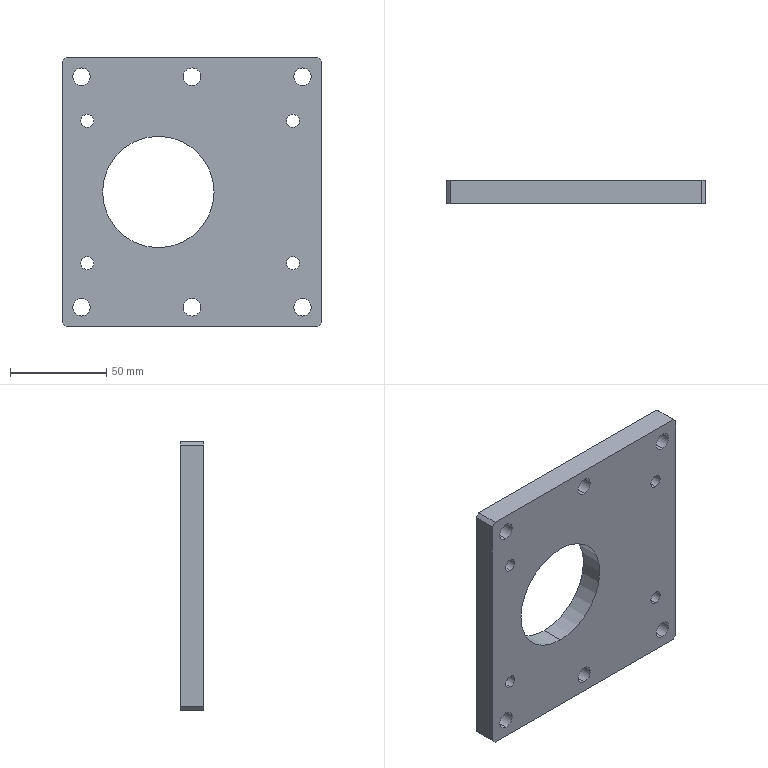Part | STEP file | 0229_201_Plate | 1 solid | 32 faces | box 135 x 12 x 140 mm | volume 188675 mm3 | cylinder 22 | plane 10 | commonest cylinder face diameters 9 x12 6.8 x8 58 x2